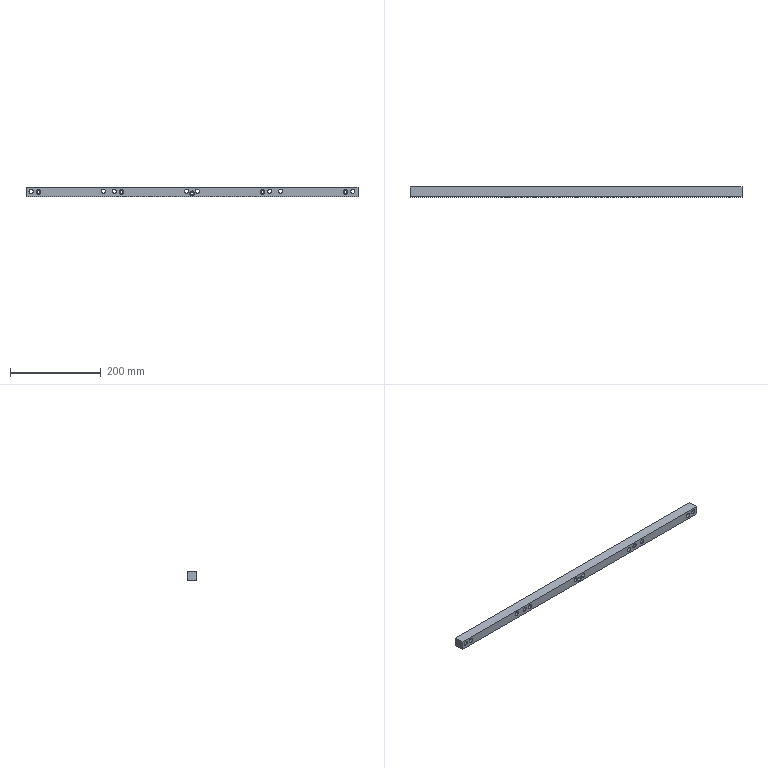Part | NX | features BREP 1 | 1 solid | 73 faces | box 731 x 22 x 20 mm | volume 305206 mm3 | cylinder 36 | cone 26 | plane 11 | commonest cylinder face diameters 8.8 x16 6.2 x10 9.5 x10